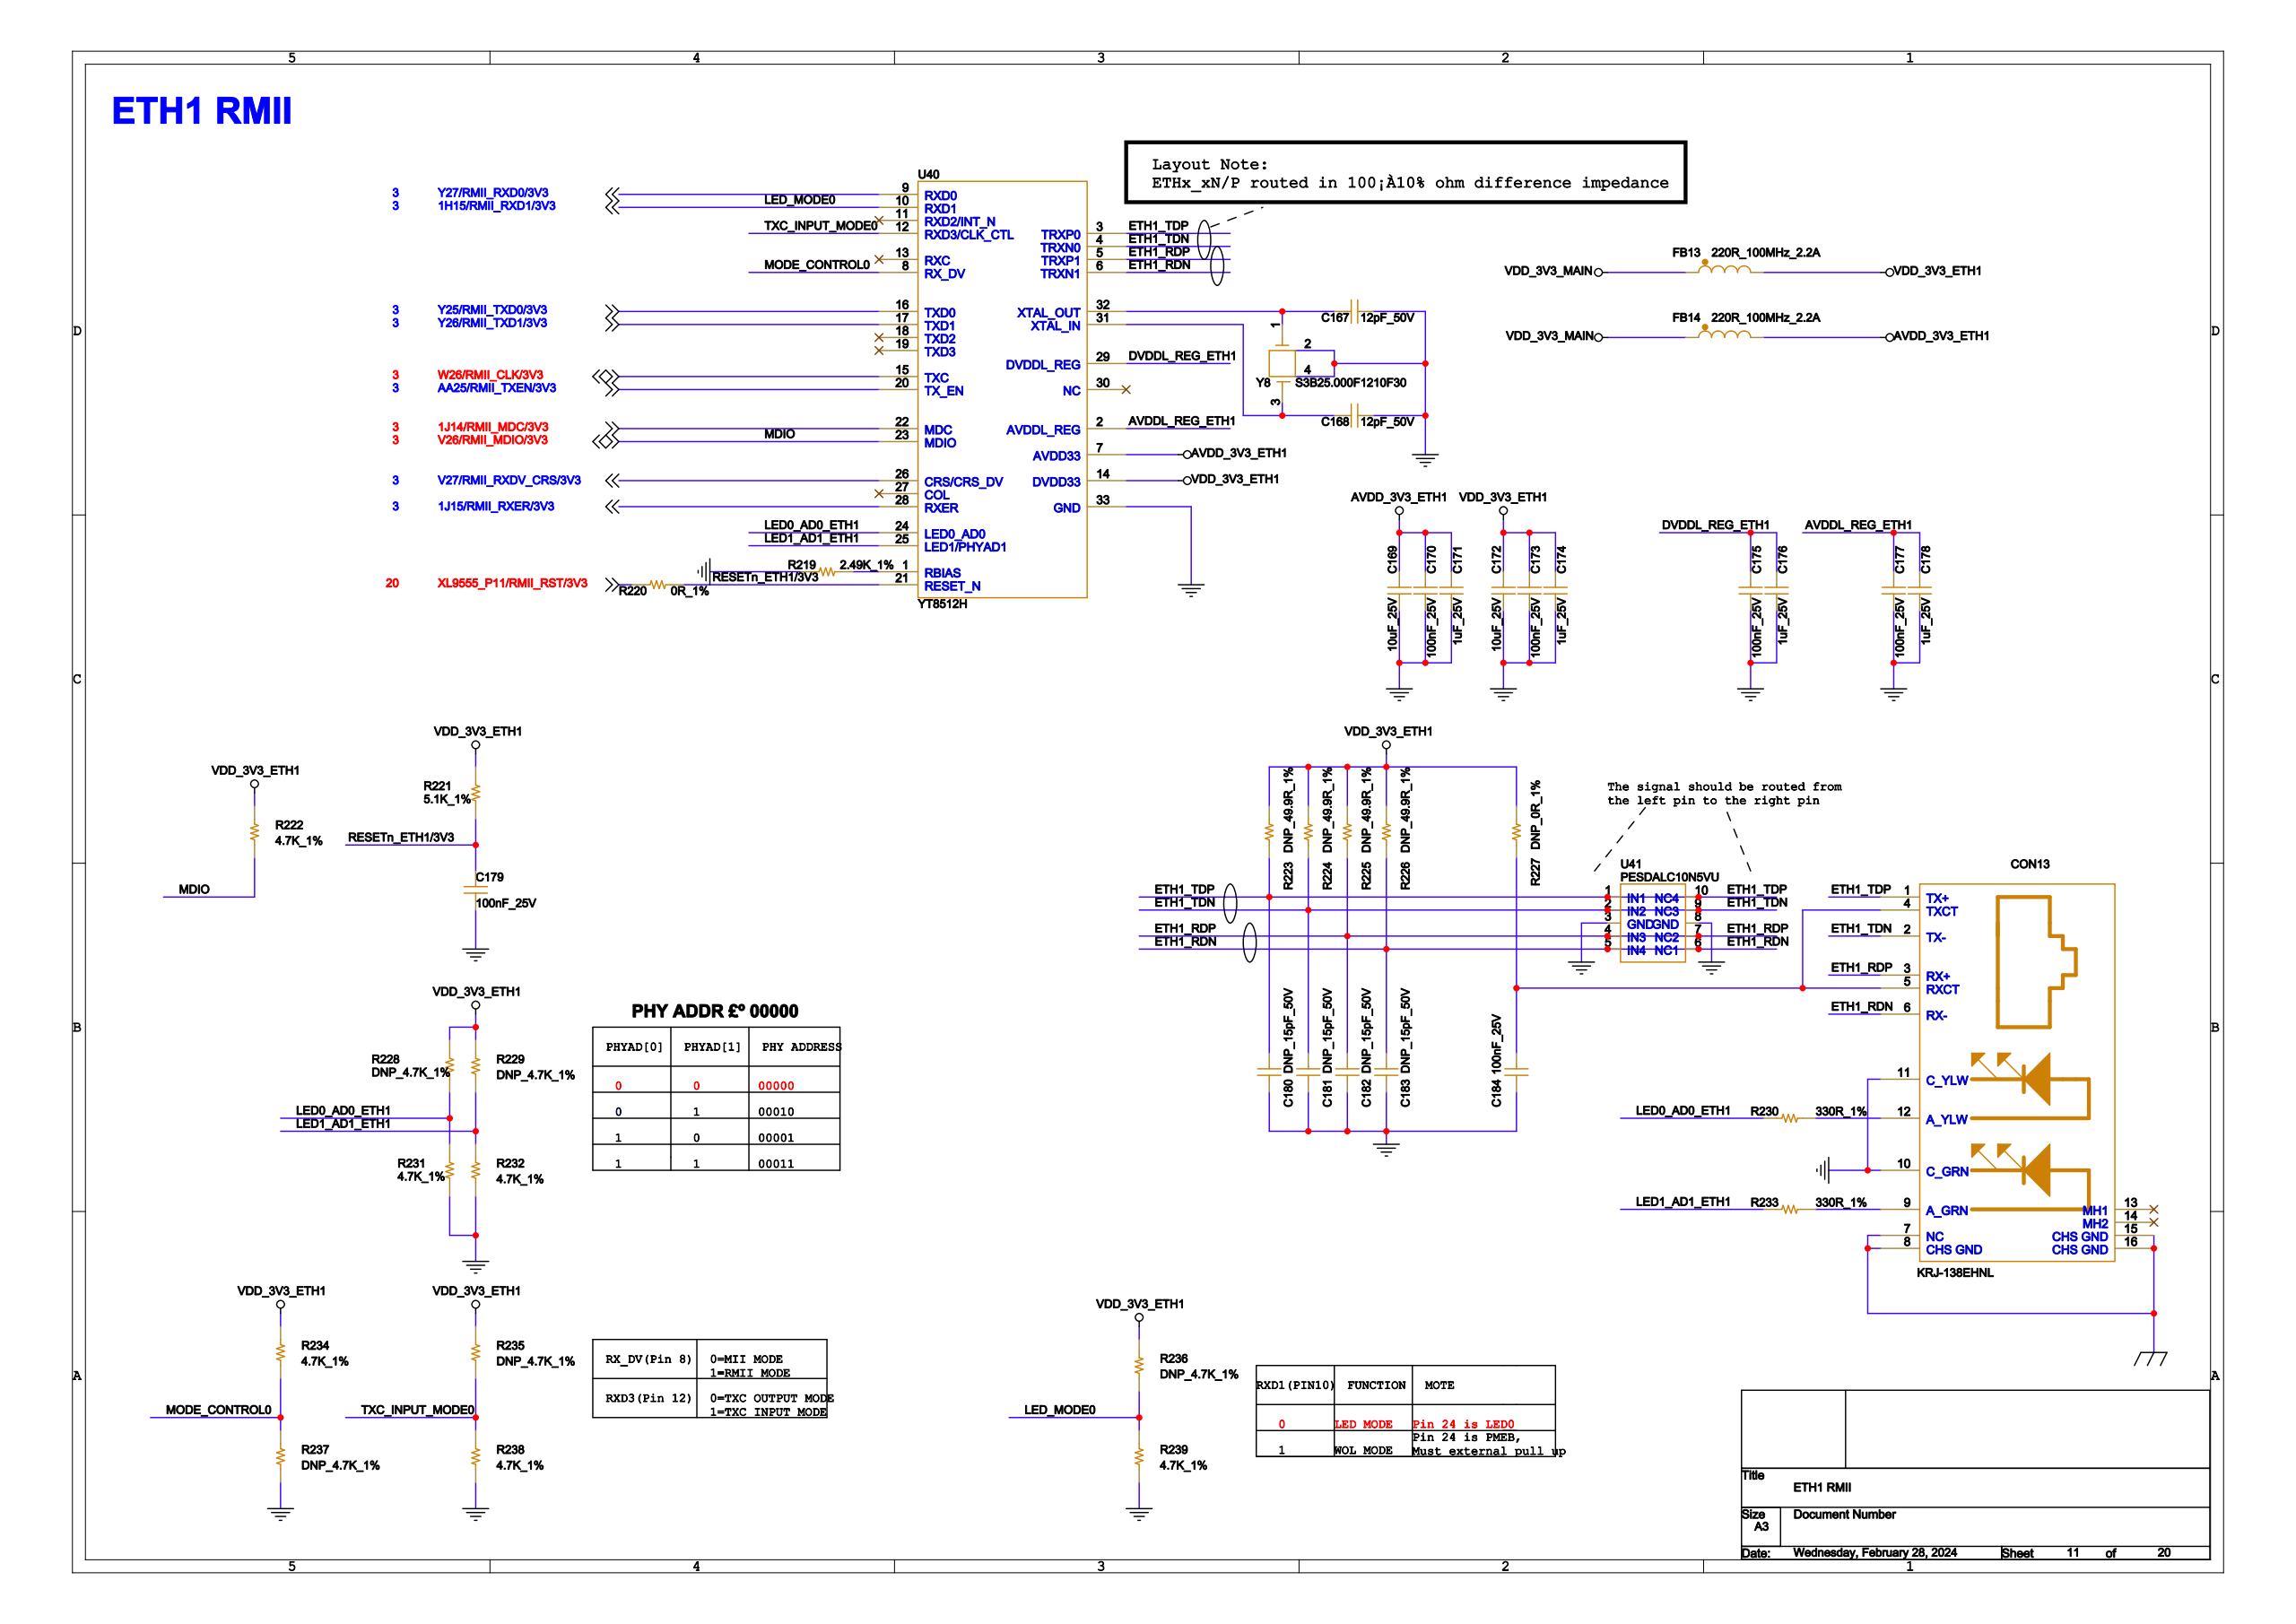Circuit board | Cadence Allegro | 1024 parts | 682 nets | one sheet of the schematic
Parts on this sheet (reference | value | footprint):
C167 | 12pF_50V | C0402
C168 | 12pF_50V | C0402
C169 | 10uF_25V | C0603
C170 | 100nF_25V | C0402
C171 | 1uF_25V | C0603
C172 | 10uF_25V | C0603
C173 | 100nF_25V | C0402
C174 | 1uF_25V | C0603
C175 | 100nF_25V | C0402
C176 | 1uF_25V | C0603
C177 | 100nF_25V | C0402
C178 | 1uF_25V | C0603
C179 | 100nF_25V | C0402
C180 | DNP_15pF_50V | C0603
C181 | DNP_15pF_50V | C0603
C182 | DNP_15pF_50V | C0603
C183 | DNP_15pF_50V | C0603
C184 | 100nF_25V | C0402
CON13 | KRJ-138EHNL | CON_YDS_13F-64GYD2PLXNL
FB13 | 220R_100MHz_2A | L0603
FB14 | 220R_100MHz_2A | L0603
R219 | 2.49K_1% | R0603
R220 | 0R_1% | R0402
R221 | 5.1K_1% | R0402
R222 | 4.7K_1% | R0402
R223 | DNP_49.9R_1% | R0603
R224 | DNP_49.9R_1% | R0603
R225 | DNP_49.9R_1% | R0603
R226 | DNP_49.9R_1% | R0603
R227 | DNP_0R_1% | R0402
R228 | DNP_4.7K_1% | R0402
R229 | DNP_4.7K_1% | R0402
R230 | 330R_1% | R0402
R231 | 4.7K_1% | R0402
R232 | 4.7K_1% | R0402
R233 | 330R_1% | R0402
R234 | 4.7K_1% | R0402
R235 | DNP_4.7K_1% | R0402
R236 | DNP_4.7K_1% | R0402
R237 | DNP_4.7K_1% | R0402
R238 | 4.7K_1% | R0402
R239 | 4.7K_1% | R0402
U40 | YT8512H | QFN32
U41 | PESDALC10N5VU | DFN-10-2510
Y8 | S3B25.000F1210F30 | SMD_3225
Nets of these parts (net: part-pin ...):
GND: C167-1 C168-1 C169-2 C170-2 C171-2 C172-2 C173-2 C174-2 C175-2 C176-2 C177-2 C178-2 C179-2 C180-2 C181-2 C182-2 C183-2 C184-2 CON13-10 CON13-11 R219-2 R231-1 R232-1 R237-2 R238-2 R239-2 U41-3 U41-8 Y8-2 Y8-4 U40-33
EGND: CON13-7 CON13-8 CON13-15 CON13-16
VDD_3V3_MAIN: FB13-1 FB14-1
N21606867: C167-2 Y8-1 U40-32
N21606869: C168-2 Y8-3 U40-31
AVDD_3V3_ETH1: C169-1 C170-1 C171-1 FB14-2 U40-7
VDD_3V3_ETH1: C172-1 C173-1 C174-1 FB13-2 R221-1 R222-1 R223-1 R224-1 R225-1 R226-1 R227-2 R228-2 R229-2 R234-2 R235-2 R236-2 U40-14
DVDDL_REG_ETH1: C175-1 C176-1 U40-29
AVDDL_REG_ETH1: C177-1 C178-1 U40-2
RESETN_ETH1/3V3: C179-1 R220-2 R221-2 U40-21
ETH1_TDP: C180-1 CON13-1 R223-2 U41-1 U41-10 U40-3
ETH1_TDN: C181-1 CON13-2 R224-2 U41-2 U41-9 U40-4
ETH1_RDP: C182-1 CON13-3 R225-2 U41-4 U41-7 U40-5
ETH1_RDN: C183-1 CON13-6 R226-2 U41-5 U41-6 U40-6
N21606388: C184-1 CON13-4 CON13-5 R227-1
1J15/RMII_RXER/3V3: U40-28
Y27/RMII_RXD0/3V3: U40-9
AA25/RMII_TXEN/3V3: U40-20
1H15/RMII_RXD1/3V3: R236-1 R239-1 U40-10
Y25/RMII_TXD0/3V3: U40-16
V27/RMII_RXDV_CRS/3V3: U40-26
Y26/RMII_TXD1/3V3: U40-17
W26/RMII_CLK/3V3: U40-15
N21606466: CON13-9 R233-2
N21606462: CON13-12 R230-2
N21607302: R219-1 U40-1
XL9555_P11/RMII_RST/3V3: R220-1
V26/RMII_MDIO/3V3: R222-2 U40-23
LED0_AD0_ETH1: R228-1 R230-1 R231-2 U40-24
LED1_AD1_ETH1: R229-1 R232-2 R233-1 U40-25
MODE_CONTROL0: R234-1 R237-1 U40-8
TXC_INPUT_MODE0: R235-1 R238-1 U40-12
1J14/RMII_MDC/3V3: U40-22